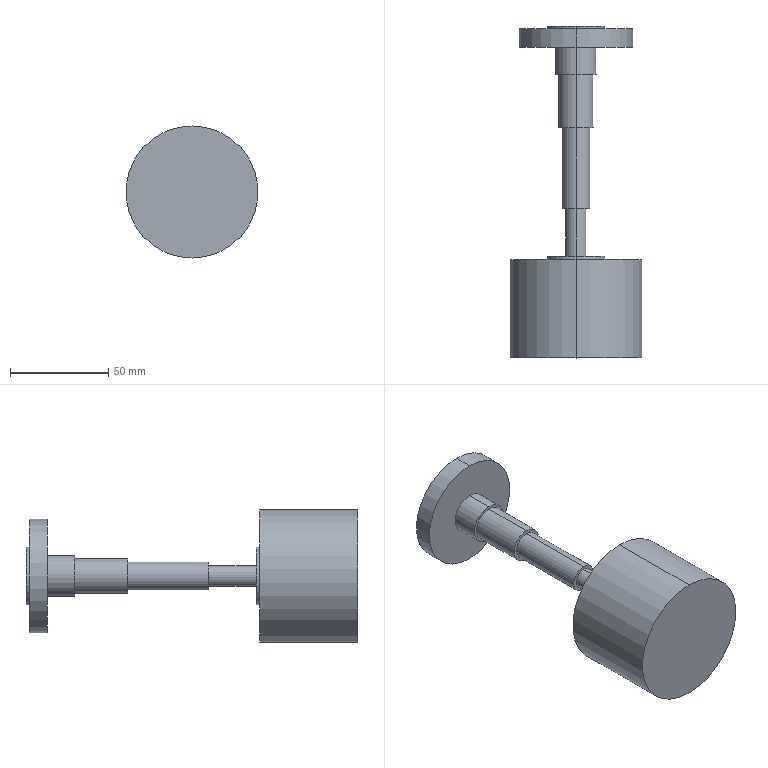Part | SolidWorks | features SavedExtBody 1 | 1 solid | 28 faces | box 67.426 x 169.265 x 67.426 mm | volume 221151 mm3 | cylinder 18 | plane 10 | commonest cylinder face diameters 29.345 x4 7.234 x2 10.656 x2 14.186 x2 17.774 x2 20.753 x2
STEP:
#1=CARTESIAN_POINT('',(0.,-304.394,79.672));
#2=VERTEX_POINT('',#1);
#3=CARTESIAN_POINT('',(0.,-304.394,50.328));
#4=VERTEX_POINT('',#3);
#5=CARTESIAN_POINT('',(0.,-304.394,65.));
#6=DIRECTION('',(0.,1.,0.));
#7=DIRECTION('',(0.,0.,1.));
#8=AXIS2_PLACEMENT_3D('',#5,#6,#7);
#9=CIRCLE('',#8,14.672);
#10=EDGE_CURVE('',#2,#4,#9,.T.);
#11=ORIENTED_EDGE('',*,*,#10,.T.);
#12=CARTESIAN_POINT('',(0.,-302.738,50.328));
#13=VERTEX_POINT('',#12);
#14=CARTESIAN_POINT('',(0.,-304.394,50.328));
#15=DIRECTION('',(0.,1.,0.));
#16=VECTOR('',#15,1000.);
#17=LINE('',#14,#16);
#18=EDGE_CURVE('',#4,#13,#17,.T.);
#19=ORIENTED_EDGE('',*,*,#18,.T.);
#20=CARTESIAN_POINT('',(0.,-302.738,79.672));
#21=VERTEX_POINT('',#20);
#22=CARTESIAN_POINT('',(0.,-302.738,65.));
#23=DIRECTION('',(0.,1.,0.));
#24=DIRECTION('',(0.,0.,1.));
#25=AXIS2_PLACEMENT_3D('',#22,#23,#24);
#26=CIRCLE('',#25,14.672);
#27=EDGE_CURVE('',#21,#13,#26,.T.);
#28=ORIENTED_EDGE('',*,*,#27,.F.);
#29=CARTESIAN_POINT('',(0.,-304.394,79.672));
#30=DIRECTION('',(0.,1.,0.));
#31=VECTOR('',#30,1000.);
#32=LINE('',#29,#31);
#33=EDGE_CURVE('',#2,#21,#32,.T.);
#34=ORIENTED_EDGE('',*,*,#33,.F.);
#35=EDGE_LOOP('',(#11,#19,#28,#34));
#36=FACE_OUTER_BOUND('',#35,.T.);
#37=CARTESIAN_POINT('',(0.,-304.394,65.));
#38=DIRECTION('',(0.,1.,0.));
#39=DIRECTION('',(0.,0.,1.));
#40=AXIS2_PLACEMENT_3D('',#37,#38,#39);
#41=CYLINDRICAL_SURFACE('',#40,14.672);
#42=ADVANCED_FACE('',(#36),#41,.T.);
#43=CARTESIAN_POINT('',(0.,-302.738,70.328));
#44=VERTEX_POINT('',#43);
#45=CARTESIAN_POINT('',(0.,-302.738,59.672));
#46=VERTEX_POINT('',#45);
#47=CARTESIAN_POINT('',(0.,-302.738,65.));
#48=DIRECTION('',(0.,1.,0.));
#49=DIRECTION('',(0.,0.,1.));
#50=AXIS2_PLACEMENT_3D('',#47,#48,#49);
#51=CIRCLE('',#50,5.328);
#52=EDGE_CURVE('',#44,#46,#51,.T.);
#53=ORIENTED_EDGE('',*,*,#52,.T.);
#54=CARTESIAN_POINT('',(0.,-278.363,59.672));
#55=VERTEX_POINT('',#54);
#56=CARTESIAN_POINT('',(0.,-304.394,59.672));
#57=DIRECTION('',(0.,1.,0.));
#58=VECTOR('',#57,1000.);
#59=LINE('',#56,#58);
#60=EDGE_CURVE('',#46,#55,#59,.T.);
#61=ORIENTED_EDGE('',*,*,#60,.T.);
#62=CARTESIAN_POINT('',(0.,-278.363,70.328));
#63=VERTEX_POINT('',#62);
#64=CARTESIAN_POINT('',(0.,-278.363,65.));
#65=DIRECTION('',(0.,1.,0.));
#66=DIRECTION('',(0.,0.,1.));
#67=AXIS2_PLACEMENT_3D('',#64,#65,#66);
#68=CIRCLE('',#67,5.328);
#69=EDGE_CURVE('',#63,#55,#68,.T.);
#70=ORIENTED_EDGE('',*,*,#69,.F.);
#71=CARTESIAN_POINT('',(0.,-304.394,70.328));
#72=DIRECTION('',(0.,1.,0.));
#73=VECTOR('',#72,1000.);
#74=LINE('',#71,#73);
#75=EDGE_CURVE('',#44,#63,#74,.T.);
#76=ORIENTED_EDGE('',*,*,#75,.F.);
#77=EDGE_LOOP('',(#53,#61,#70,#76));
#78=FACE_OUTER_BOUND('',#77,.T.);
#79=CARTESIAN_POINT('',(0.,-304.394,65.));
#80=DIRECTION('',(0.,1.,0.));
#81=DIRECTION('',(0.,0.,1.));
#82=AXIS2_PLACEMENT_3D('',#79,#80,#81);
#83=CYLINDRICAL_SURFACE('',#82,5.328);
#84=ADVANCED_FACE('',(#78),#83,.T.);
#85=CARTESIAN_POINT('',(0.,-278.363,72.093));
#86=VERTEX_POINT('',#85);
#87=CARTESIAN_POINT('',(0.,-278.363,57.907));
#88=VERTEX_POINT('',#87);
#89=CARTESIAN_POINT('',(0.,-278.363,65.));
#90=DIRECTION('',(0.,1.,0.));
#91=DIRECTION('',(0.,0.,1.));
#92=AXIS2_PLACEMENT_3D('',#89,#90,#91);
#93=CIRCLE('',#92,7.093);
#94=EDGE_CURVE('',#86,#88,#93,.T.);
#95=ORIENTED_EDGE('',*,*,#94,.T.);
#96=CARTESIAN_POINT('',(0.,-237.148,57.907));
#97=VERTEX_POINT('',#96);
#98=CARTESIAN_POINT('',(0.,-304.394,57.907));
#99=DIRECTION('',(0.,1.,0.));
#100=VECTOR('',#99,1000.);
#101=LINE('',#98,#100);
#102=EDGE_CURVE('',#88,#97,#101,.T.);
#103=ORIENTED_EDGE('',*,*,#102,.T.);
#104=CARTESIAN_POINT('',(0.,-237.148,72.093));
#105=VERTEX_POINT('',#104);
#106=CARTESIAN_POINT('',(0.,-237.148,65.));
#107=DIRECTION('',(0.,1.,0.));
#108=DIRECTION('',(0.,0.,1.));
#109=AXIS2_PLACEMENT_3D('',#106,#107,#108);
#110=CIRCLE('',#109,7.093);
#111=EDGE_CURVE('',#105,#97,#110,.T.);
#112=ORIENTED_EDGE('',*,*,#111,.F.);
#113=CARTESIAN_POINT('',(0.,-304.394,72.093));
#114=DIRECTION('',(0.,1.,0.));
#115=VECTOR('',#114,1000.);
#116=LINE('',#113,#115);
#117=EDGE_CURVE('',#86,#105,#116,.T.);
#118=ORIENTED_EDGE('',*,*,#117,.F.);
#119=EDGE_LOOP('',(#95,#103,#112,#118));
#120=FACE_OUTER_BOUND('',#119,.T.);
#121=CARTESIAN_POINT('',(0.,-304.394,65.));
#122=DIRECTION('',(0.,1.,0.));
#123=DIRECTION('',(0.,0.,1.));
#124=AXIS2_PLACEMENT_3D('',#121,#122,#123);
#125=CYLINDRICAL_SURFACE('',#124,7.093);
#126=ADVANCED_FACE('',(#120),#125,.T.);
#127=CARTESIAN_POINT('',(0.,-237.148,73.887));
#128=VERTEX_POINT('',#127);
#129=CARTESIAN_POINT('',(0.,-237.148,56.113));
#130=VERTEX_POINT('',#129);
#131=CARTESIAN_POINT('',(0.,-237.148,65.));
#132=DIRECTION('',(0.,1.,0.));
#133=DIRECTION('',(0.,0.,1.));
#134=AXIS2_PLACEMENT_3D('',#131,#132,#133);
#135=CIRCLE('',#134,8.887);
#136=EDGE_CURVE('',#128,#130,#135,.T.);
#137=ORIENTED_EDGE('',*,*,#136,.T.);
#138=CARTESIAN_POINT('',(0.,-210.021,56.113));
#139=VERTEX_POINT('',#138);
#140=CARTESIAN_POINT('',(0.,-304.394,56.113));
#141=DIRECTION('',(0.,1.,0.));
#142=VECTOR('',#141,1000.);
#143=LINE('',#140,#142);
#144=EDGE_CURVE('',#130,#139,#143,.T.);
#145=ORIENTED_EDGE('',*,*,#144,.T.);
#146=CARTESIAN_POINT('',(0.,-210.021,73.887));
#147=VERTEX_POINT('',#146);
#148=CARTESIAN_POINT('',(0.,-210.021,65.));
#149=DIRECTION('',(0.,1.,0.));
#150=DIRECTION('',(0.,0.,1.));
#151=AXIS2_PLACEMENT_3D('',#148,#149,#150);
#152=CIRCLE('',#151,8.887);
#153=EDGE_CURVE('',#147,#139,#152,.T.);
#154=ORIENTED_EDGE('',*,*,#153,.F.);
#155=CARTESIAN_POINT('',(0.,-304.394,73.887));
#156=DIRECTION('',(0.,1.,0.));
#157=VECTOR('',#156,1000.);
#158=LINE('',#155,#157);
#159=EDGE_CURVE('',#128,#147,#158,.T.);
#160=ORIENTED_EDGE('',*,*,#159,.F.);
#161=EDGE_LOOP('',(#137,#145,#154,#160));
#162=FACE_OUTER_BOUND('',#161,.T.);
#163=CARTESIAN_POINT('',(0.,-304.394,65.));
#164=DIRECTION('',(0.,1.,0.));
#165=DIRECTION('',(0.,0.,1.));
#166=AXIS2_PLACEMENT_3D('',#163,#164,#165);
#167=CYLINDRICAL_SURFACE('',#166,8.887);
#168=ADVANCED_FACE('',(#162),#167,.T.);
#169=CARTESIAN_POINT('',(0.,-210.021,75.377));
#170=VERTEX_POINT('',#169);
#171=CARTESIAN_POINT('',(0.,-210.021,54.623));
#172=VERTEX_POINT('',#171);
#173=CARTESIAN_POINT('',(0.,-210.021,65.));
#174=DIRECTION('',(0.,1.,0.));
#175=DIRECTION('',(0.,0.,1.));
#176=AXIS2_PLACEMENT_3D('',#173,#174,#175);
#177=CIRCLE('',#176,10.377);
#178=EDGE_CURVE('',#170,#172,#177,.T.);
#179=ORIENTED_EDGE('',*,*,#178,.T.);
#180=CARTESIAN_POINT('',(0.,-196.144,54.623));
#181=VERTEX_POINT('',#180);
#182=CARTESIAN_POINT('',(0.,-304.394,54.623));
#183=DIRECTION('',(0.,1.,0.));
#184=VECTOR('',#183,1000.);
#185=LINE('',#182,#184);
#186=EDGE_CURVE('',#172,#181,#185,.T.);
#187=ORIENTED_EDGE('',*,*,#186,.T.);
#188=CARTESIAN_POINT('',(0.,-196.144,75.377));
#189=VERTEX_POINT('',#188);
#190=CARTESIAN_POINT('',(0.,-196.144,65.));
#191=DIRECTION('',(0.,1.,0.));
#192=DIRECTION('',(0.,0.,1.));
#193=AXIS2_PLACEMENT_3D('',#190,#191,#192);
#194=CIRCLE('',#193,10.377);
#195=EDGE_CURVE('',#189,#181,#194,.T.);
#196=ORIENTED_EDGE('',*,*,#195,.F.);
#197=CARTESIAN_POINT('',(0.,-304.394,75.377));
#198=DIRECTION('',(0.,1.,0.));
#199=VECTOR('',#198,1000.);
#200=LINE('',#197,#199);
#201=EDGE_CURVE('',#170,#189,#200,.T.);
#202=ORIENTED_EDGE('',*,*,#201,.F.);
#203=EDGE_LOOP('',(#179,#187,#196,#202));
#204=FACE_OUTER_BOUND('',#203,.T.);
#205=CARTESIAN_POINT('',(0.,-304.394,65.));
#206=DIRECTION('',(0.,1.,0.));
#207=DIRECTION('',(0.,0.,1.));
#208=AXIS2_PLACEMENT_3D('',#205,#206,#207);
#209=CYLINDRICAL_SURFACE('',#208,10.377);
#210=ADVANCED_FACE('',(#204),#209,.T.);
#211=CARTESIAN_POINT('',(0.,-196.144,93.981));
#212=VERTEX_POINT('',#211);
#213=CARTESIAN_POINT('',(0.,-196.144,36.019));
#214=VERTEX_POINT('',#213);
#215=CARTESIAN_POINT('',(0.,-196.144,65.));
#216=DIRECTION('',(0.,1.,0.));
#217=DIRECTION('',(0.,0.,1.));
#218=AXIS2_PLACEMENT_3D('',#215,#216,#217);
#219=CIRCLE('',#218,28.981);
#220=EDGE_CURVE('',#212,#214,#219,.T.);
#221=ORIENTED_EDGE('',*,*,#220,.T.);
#222=CARTESIAN_POINT('',(0.,-186.774,36.019));
#223=VERTEX_POINT('',#222);
#224=CARTESIAN_POINT('',(0.,-304.394,36.019));
#225=DIRECTION('',(0.,1.,0.));
#226=VECTOR('',#225,1000.);
#227=LINE('',#224,#226);
#228=EDGE_CURVE('',#214,#223,#227,.T.);
#229=ORIENTED_EDGE('',*,*,#228,.T.);
#230=CARTESIAN_POINT('',(0.,-186.774,93.981));
#231=VERTEX_POINT('',#230);
#232=CARTESIAN_POINT('',(0.,-186.774,65.));
#233=DIRECTION('',(0.,1.,0.));
#234=DIRECTION('',(0.,0.,1.));
#235=AXIS2_PLACEMENT_3D('',#232,#233,#234);
#236=CIRCLE('',#235,28.981);
#237=EDGE_CURVE('',#231,#223,#236,.T.);
#238=ORIENTED_EDGE('',*,*,#237,.F.);
#239=CARTESIAN_POINT('',(0.,-304.394,93.981));
#240=DIRECTION('',(0.,1.,0.));
#241=VECTOR('',#240,1000.);
#242=LINE('',#239,#241);
#243=EDGE_CURVE('',#212,#231,#242,.T.);
#244=ORIENTED_EDGE('',*,*,#243,.F.);
#245=EDGE_LOOP('',(#221,#229,#238,#244));
#246=FACE_OUTER_BOUND('',#245,.T.);
#247=CARTESIAN_POINT('',(0.,-304.394,65.));
#248=DIRECTION('',(0.,1.,0.));
#249=DIRECTION('',(0.,0.,1.));
#250=AXIS2_PLACEMENT_3D('',#247,#248,#249);
#251=CYLINDRICAL_SURFACE('',#250,28.981);
#252=ADVANCED_FACE('',(#246),#251,.T.);
#253=CARTESIAN_POINT('',(0.,-186.774,79.672));
#254=VERTEX_POINT('',#253);
#255=CARTESIAN_POINT('',(0.,-186.774,50.328));
#256=VERTEX_POINT('',#255);
#257=CARTESIAN_POINT('',(0.,-186.774,65.));
#258=DIRECTION('',(0.,1.,0.));
#259=DIRECTION('',(0.,0.,1.));
#260=AXIS2_PLACEMENT_3D('',#257,#258,#259);
#261=CIRCLE('',#260,14.672);
#262=EDGE_CURVE('',#254,#256,#261,.T.);
#263=ORIENTED_EDGE('',*,*,#262,.T.);
#264=CARTESIAN_POINT('',(0.,-185.285,50.328));
#265=VERTEX_POINT('',#264);
#266=CARTESIAN_POINT('',(0.,-304.394,50.328));
#267=DIRECTION('',(0.,1.,0.));
#268=VECTOR('',#267,1000.);
#269=LINE('',#266,#268);
#270=EDGE_CURVE('',#256,#265,#269,.T.);
#271=ORIENTED_EDGE('',*,*,#270,.T.);
#272=CARTESIAN_POINT('',(0.,-185.285,79.672));
#273=VERTEX_POINT('',#272);
#274=CARTESIAN_POINT('',(0.,-185.285,65.));
#275=DIRECTION('',(0.,1.,0.));
#276=DIRECTION('',(0.,0.,1.));
#277=AXIS2_PLACEMENT_3D('',#274,#275,#276);
#278=CIRCLE('',#277,14.672);
#279=EDGE_CURVE('',#273,#265,#278,.T.);
#280=ORIENTED_EDGE('',*,*,#279,.F.);
#281=CARTESIAN_POINT('',(0.,-304.394,79.672));
#282=DIRECTION('',(0.,1.,0.));
#283=VECTOR('',#282,1000.);
#284=LINE('',#281,#283);
#285=EDGE_CURVE('',#254,#273,#284,.T.);
#286=ORIENTED_EDGE('',*,*,#285,.F.);
#287=EDGE_LOOP('',(#263,#271,#280,#286));
#288=FACE_OUTER_BOUND('',#287,.T.);
#289=CARTESIAN_POINT('',(0.,-304.394,65.));
#290=DIRECTION('',(0.,1.,0.));
#291=DIRECTION('',(0.,0.,1.));
#292=AXIS2_PLACEMENT_3D('',#289,#290,#291);
#293=CYLINDRICAL_SURFACE('',#292,14.672);
#294=ADVANCED_FACE('',(#288),#293,.T.);
#295=CARTESIAN_POINT('',(0.,-304.394,61.383));
#296=VERTEX_POINT('',#295);
#297=CARTESIAN_POINT('',(0.,-304.394,68.617));
#298=VERTEX_POINT('',#297);
#299=CARTESIAN_POINT('',(0.,-304.394,65.));
#300=DIRECTION('',(0.,1.,0.));
#301=DIRECTION('',(0.,0.,1.));
#302=AXIS2_PLACEMENT_3D('',#299,#300,#301);
#303=CIRCLE('',#302,3.617);
#304=EDGE_CURVE('',#296,#298,#303,.T.);
#305=ORIENTED_EDGE('',*,*,#304,.F.);
#306=CARTESIAN_POINT('',(0.,-185.285,61.383));
#307=VERTEX_POINT('',#306);
#308=CARTESIAN_POINT('',(0.,-304.394,61.383));
#309=DIRECTION('',(0.,1.,0.));
#310=VECTOR('',#309,1000.);
#311=LINE('',#308,#310);
#312=EDGE_CURVE('',#296,#307,#311,.T.);
#313=ORIENTED_EDGE('',*,*,#312,.T.);
#314=CARTESIAN_POINT('',(0.,-185.285,68.617));
#315=VERTEX_POINT('',#314);
#316=CARTESIAN_POINT('',(0.,-185.285,65.));
#317=DIRECTION('',(0.,1.,0.));
#318=DIRECTION('',(0.,0.,1.));
#319=AXIS2_PLACEMENT_3D('',#316,#317,#318);
#320=CIRCLE('',#319,3.617);
#321=EDGE_CURVE('',#307,#315,#320,.T.);
#322=ORIENTED_EDGE('',*,*,#321,.T.);
#323=CARTESIAN_POINT('',(0.,-304.394,68.617));
#324=DIRECTION('',(0.,1.,0.));
#325=VECTOR('',#324,1000.);
#326=LINE('',#323,#325);
#327=EDGE_CURVE('',#298,#315,#326,.T.);
#328=ORIENTED_EDGE('',*,*,#327,.F.);
#329=EDGE_LOOP('',(#305,#313,#322,#328));
#330=FACE_OUTER_BOUND('',#329,.T.);
#331=CARTESIAN_POINT('',(0.,-304.394,65.));
#332=DIRECTION('',(0.,1.,0.));
#333=DIRECTION('',(0.,0.,1.));
#334=AXIS2_PLACEMENT_3D('',#331,#332,#333);
#335=CYLINDRICAL_SURFACE('',#334,3.617);
#336=ADVANCED_FACE('',(#330),#335,.F.);
#337=CARTESIAN_POINT('',(0.,-354.549,98.713));
#338=VERTEX_POINT('',#337);
#339=CARTESIAN_POINT('',(0.,-354.549,31.287));
#340=VERTEX_POINT('',#339);
#341=CARTESIAN_POINT('',(0.,-354.549,65.));
#342=DIRECTION('',(0.,1.,0.));
#343=DIRECTION('',(0.,0.,1.));
#344=AXIS2_PLACEMENT_3D('',#341,#342,#343);
#345=CIRCLE('',#344,33.713);
#346=EDGE_CURVE('',#338,#340,#345,.T.);
#347=ORIENTED_EDGE('',*,*,#346,.T.);
#348=CARTESIAN_POINT('',(0.,-304.394,31.287));
#349=VERTEX_POINT('',#348);
#350=CARTESIAN_POINT('',(0.,-304.394,31.287));
#351=DIRECTION('',(0.,1.,0.));
#352=VECTOR('',#351,1000.);
#353=LINE('',#350,#352);
#354=EDGE_CURVE('',#340,#349,#353,.T.);
#355=ORIENTED_EDGE('',*,*,#354,.T.);
#356=CARTESIAN_POINT('',(0.,-304.394,98.713));
#357=VERTEX_POINT('',#356);
#358=CARTESIAN_POINT('',(0.,-304.394,65.));
#359=DIRECTION('',(0.,1.,0.));
#360=DIRECTION('',(0.,0.,1.));
#361=AXIS2_PLACEMENT_3D('',#358,#359,#360);
#362=CIRCLE('',#361,33.713);
#363=EDGE_CURVE('',#357,#349,#362,.T.);
#364=ORIENTED_EDGE('',*,*,#363,.F.);
#365=CARTESIAN_POINT('',(0.,-304.394,98.713));
#366=DIRECTION('',(0.,1.,0.));
#367=VECTOR('',#366,1000.);
#368=LINE('',#365,#367);
#369=EDGE_CURVE('',#338,#357,#368,.T.);
#370=ORIENTED_EDGE('',*,*,#369,.F.);
#371=EDGE_LOOP('',(#347,#355,#364,#370));
#372=FACE_OUTER_BOUND('',#371,.T.);
#373=CARTESIAN_POINT('',(0.,-304.394,65.));
#374=DIRECTION('',(0.,1.,0.));
#375=DIRECTION('',(0.,0.,1.));
#376=AXIS2_PLACEMENT_3D('',#373,#374,#375);
#377=CYLINDRICAL_SURFACE('',#376,33.713);
#378=ADVANCED_FACE('',(#372),#377,.T.);
#379=ORIENTED_EDGE('',*,*,#354,.F.);
#380=CARTESIAN_POINT('',(0.,-354.549,65.));
#381=DIRECTION('',(0.,1.,0.));
#382=DIRECTION('',(0.,0.,1.));
#383=AXIS2_PLACEMENT_3D('',#380,#381,#382);
#384=CIRCLE('',#383,33.713);
#385=EDGE_CURVE('',#340,#338,#384,.T.);
#386=ORIENTED_EDGE('',*,*,#385,.T.);
#387=ORIENTED_EDGE('',*,*,#369,.T.);
#388=CARTESIAN_POINT('',(0.,-304.394,65.));
#389=DIRECTION('',(0.,1.,0.));
#390=DIRECTION('',(0.,0.,1.));
#391=AXIS2_PLACEMENT_3D('',#388,#389,#390);
#392=CIRCLE('',#391,33.713);
#393=EDGE_CURVE('',#349,#357,#392,.T.);
#394=ORIENTED_EDGE('',*,*,#393,.F.);
#395=EDGE_LOOP('',(#379,#386,#387,#394));
#396=FACE_OUTER_BOUND('',#395,.T.);
#397=CARTESIAN_POINT('',(0.,-304.394,65.));
#398=DIRECTION('',(0.,1.,0.));
#399=DIRECTION('',(0.,0.,1.));
#400=AXIS2_PLACEMENT_3D('',#397,#398,#399);
#401=CYLINDRICAL_SURFACE('',#400,33.713);
#402=ADVANCED_FACE('',(#396),#401,.T.);
#403=ORIENTED_EDGE('',*,*,#346,.F.);
#404=ORIENTED_EDGE('',*,*,#385,.F.);
#405=EDGE_LOOP('',(#403,#404));
#406=FACE_OUTER_BOUND('',#405,.T.);
#407=CARTESIAN_POINT('',(-33.713,-354.549,65.));
#408=DIRECTION('',(0.,-1.,0.));
#409=DIRECTION('',(0.,0.,-1.));
#410=AXIS2_PLACEMENT_3D('',#407,#408,#409);
#411=PLANE('',#410);
#412=ADVANCED_FACE('',(#406),#411,.T.);
#413=CARTESIAN_POINT('',(0.,-304.394,65.));
#414=DIRECTION('',(0.,1.,0.));
#415=DIRECTION('',(0.,0.,1.));
#416=AXIS2_PLACEMENT_3D('',#413,#414,#415);
#417=CIRCLE('',#416,3.617);
#418=EDGE_CURVE('',#298,#296,#417,.T.);
#419=ORIENTED_EDGE('',*,*,#418,.T.);
#420=ORIENTED_EDGE('',*,*,#304,.T.);
#421=EDGE_LOOP('',(#419,#420));
#422=FACE_OUTER_BOUND('',#421,.T.);
#423=CARTESIAN_POINT('',(-3.617,-304.394,65.));
#424=DIRECTION('',(0.,1.,0.));
#425=DIRECTION('',(0.,0.,1.));
#426=AXIS2_PLACEMENT_3D('',#423,#424,#425);
#427=PLANE('',#426);
#428=ADVANCED_FACE('',(#422),#427,.T.);
#429=ORIENTED_EDGE('',*,*,#312,.F.);
#430=ORIENTED_EDGE('',*,*,#418,.F.);
#431=ORIENTED_EDGE('',*,*,#327,.T.);
#432=CARTESIAN_POINT('',(0.,-185.285,65.));
#433=DIRECTION('',(0.,1.,0.));
#434=DIRECTION('',(0.,0.,1.));
#435=AXIS2_PLACEMENT_3D('',#432,#433,#434);
#436=CIRCLE('',#435,3.617);
#437=EDGE_CURVE('',#315,#307,#436,.T.);
#438=ORIENTED_EDGE('',*,*,#437,.T.);
#439=EDGE_LOOP('',(#429,#430,#431,#438));
#440=FACE_OUTER_BOUND('',#439,.T.);
#441=CARTESIAN_POINT('',(0.,-304.394,65.));
#442=DIRECTION('',(0.,1.,0.));
#443=DIRECTION('',(0.,0.,1.));
#444=AXIS2_PLACEMENT_3D('',#441,#442,#443);
#445=CYLINDRICAL_SURFACE('',#444,3.617);
#446=ADVANCED_FACE('',(#440),#445,.F.);
#447=ORIENTED_EDGE('',*,*,#279,.T.);
#448=CARTESIAN_POINT('',(0.,-185.285,65.));
#449=DIRECTION('',(0.,1.,0.));
#450=DIRECTION('',(0.,0.,1.));
#451=AXIS2_PLACEMENT_3D('',#448,#449,#450);
#452=CIRCLE('',#451,14.672);
#453=EDGE_CURVE('',#265,#273,#452,.T.);
#454=ORIENTED_EDGE('',*,*,#453,.T.);
#455=EDGE_LOOP('',(#447,#454));
#456=FACE_OUTER_BOUND('',#455,.T.);
#457=ORIENTED_EDGE('',*,*,#437,.F.);
#458=ORIENTED_EDGE('',*,*,#321,.F.);
#459=EDGE_LOOP('',(#457,#458));
#460=FACE_BOUND('',#459,.T.);
#461=CARTESIAN_POINT('',(-12.5,-185.285,65.));
#462=DIRECTION('',(0.,1.,0.));
#463=DIRECTION('',(0.,0.,1.));
#464=AXIS2_PLACEMENT_3D('',#461,#462,#463);
#465=PLANE('',#464);
#466=ADVANCED_FACE('',(#456,#460),#465,.T.);
#467=ORIENTED_EDGE('',*,*,#270,.F.);
#468=CARTESIAN_POINT('',(0.,-186.774,65.));
#469=DIRECTION('',(0.,1.,0.));
#470=DIRECTION('',(0.,0.,1.));
#471=AXIS2_PLACEMENT_3D('',#468,#469,#470);
#472=CIRCLE('',#471,14.672);
#473=EDGE_CURVE('',#256,#254,#472,.T.);
#474=ORIENTED_EDGE('',*,*,#473,.T.);
#475=ORIENTED_EDGE('',*,*,#285,.T.);
#476=ORIENTED_EDGE('',*,*,#453,.F.);
#477=EDGE_LOOP('',(#467,#474,#475,#476));
#478=FACE_OUTER_BOUND('',#477,.T.);
#479=CARTESIAN_POINT('',(0.,-304.394,65.));
#480=DIRECTION('',(0.,1.,0.));
#481=DIRECTION('',(0.,0.,1.));
#482=AXIS2_PLACEMENT_3D('',#479,#480,#481);
#483=CYLINDRICAL_SURFACE('',#482,14.672);
#484=ADVANCED_FACE('',(#478),#483,.T.);
#485=ORIENTED_EDGE('',*,*,#237,.T.);
#486=CARTESIAN_POINT('',(0.,-186.774,65.));
#487=DIRECTION('',(0.,1.,0.));
#488=DIRECTION('',(0.,0.,1.));
#489=AXIS2_PLACEMENT_3D('',#486,#487,#488);
#490=CIRCLE('',#489,28.981);
#491=EDGE_CURVE('',#223,#231,#490,.T.);
#492=ORIENTED_EDGE('',*,*,#491,.T.);
#493=EDGE_LOOP('',(#485,#492));
#494=FACE_OUTER_BOUND('',#493,.T.);
#495=ORIENTED_EDGE('',*,*,#262,.F.);
#496=ORIENTED_EDGE('',*,*,#473,.F.);
#497=EDGE_LOOP('',(#495,#496));
#498=FACE_BOUND('',#497,.T.);
#499=CARTESIAN_POINT('',(-14.672,-186.774,65.));
#500=DIRECTION('',(0.,1.,0.));
#501=DIRECTION('',(0.,0.,1.));
#502=AXIS2_PLACEMENT_3D('',#499,#500,#501);
#503=PLANE('',#502);
#504=ADVANCED_FACE('',(#494,#498),#503,.T.);
#505=ORIENTED_EDGE('',*,*,#228,.F.);
#506=CARTESIAN_POINT('',(0.,-196.144,65.));
#507=DIRECTION('',(0.,1.,0.));
#508=DIRECTION('',(0.,0.,1.));
#509=AXIS2_PLACEMENT_3D('',#506,#507,#508);
#510=CIRCLE('',#509,28.981);
#511=EDGE_CURVE('',#214,#212,#510,.T.);
#512=ORIENTED_EDGE('',*,*,#511,.T.);
#513=ORIENTED_EDGE('',*,*,#243,.T.);
#514=ORIENTED_EDGE('',*,*,#491,.F.);
#515=EDGE_LOOP('',(#505,#512,#513,#514));
#516=FACE_OUTER_BOUND('',#515,.T.);
#517=CARTESIAN_POINT('',(0.,-304.394,65.));
#518=DIRECTION('',(0.,1.,0.));
#519=DIRECTION('',(0.,0.,1.));
#520=AXIS2_PLACEMENT_3D('',#517,#518,#519);
#521=CYLINDRICAL_SURFACE('',#520,28.981);
#522=ADVANCED_FACE('',(#516),#521,.T.);
#523=ORIENTED_EDGE('',*,*,#195,.T.);
#524=CARTESIAN_POINT('',(0.,-196.144,65.));
#525=DIRECTION('',(0.,1.,0.));
#526=DIRECTION('',(0.,0.,1.));
#527=AXIS2_PLACEMENT_3D('',#524,#525,#526);
#528=CIRCLE('',#527,10.377);
#529=EDGE_CURVE('',#181,#189,#528,.T.);
#530=ORIENTED_EDGE('',*,*,#529,.T.);
#531=EDGE_LOOP('',(#523,#530));
#532=FACE_BOUND('',#531,.T.);
#533=ORIENTED_EDGE('',*,*,#220,.F.);
#534=ORIENTED_EDGE('',*,*,#511,.F.);
#535=EDGE_LOOP('',(#533,#534));
#536=FACE_OUTER_BOUND('',#535,.T.);
#537=CARTESIAN_POINT('',(-28.981,-196.144,65.));
#538=DIRECTION('',(0.,-1.,0.));
#539=DIRECTION('',(0.,0.,-1.));
#540=AXIS2_PLACEMENT_3D('',#537,#538,#539);
#541=PLANE('',#540);
#542=ADVANCED_FACE('',(#532,#536),#541,.T.);
#543=ORIENTED_EDGE('',*,*,#186,.F.);
#544=CARTESIAN_POINT('',(0.,-210.021,65.));
#545=DIRECTION('',(0.,1.,0.));
#546=DIRECTION('',(0.,0.,1.));
#547=AXIS2_PLACEMENT_3D('',#544,#545,#546);
#548=CIRCLE('',#547,10.377);
#549=EDGE_CURVE('',#172,#170,#548,.T.);
#550=ORIENTED_EDGE('',*,*,#549,.T.);
#551=ORIENTED_EDGE('',*,*,#201,.T.);
#552=ORIENTED_EDGE('',*,*,#529,.F.);
#553=EDGE_LOOP('',(#543,#550,#551,#552));
#554=FACE_OUTER_BOUND('',#553,.T.);
#555=CARTESIAN_POINT('',(0.,-304.394,65.));
#556=DIRECTION('',(0.,1.,0.));
#557=DIRECTION('',(0.,0.,1.));
#558=AXIS2_PLACEMENT_3D('',#555,#556,#557);
#559=CYLINDRICAL_SURFACE('',#558,10.377);
#560=ADVANCED_FACE('',(#554),#559,.T.);
#561=ORIENTED_EDGE('',*,*,#153,.T.);
#562=CARTESIAN_POINT('',(0.,-210.021,65.));
#563=DIRECTION('',(0.,1.,0.));
#564=DIRECTION('',(0.,0.,1.));
#565=AXIS2_PLACEMENT_3D('',#562,#563,#564);
#566=CIRCLE('',#565,8.887);
#567=EDGE_CURVE('',#139,#147,#566,.T.);
#568=ORIENTED_EDGE('',*,*,#567,.T.);
#569=EDGE_LOOP('',(#561,#568));
#570=FACE_BOUND('',#569,.T.);
#571=ORIENTED_EDGE('',*,*,#178,.F.);
#572=ORIENTED_EDGE('',*,*,#549,.F.);
#573=EDGE_LOOP('',(#571,#572));
#574=FACE_OUTER_BOUND('',#573,.T.);
#575=CARTESIAN_POINT('',(-10.377,-210.021,65.));
#576=DIRECTION('',(0.,-1.,0.));
#577=DIRECTION('',(0.,0.,-1.));
#578=AXIS2_PLACEMENT_3D('',#575,#576,#577);
#579=PLANE('',#578);
#580=ADVANCED_FACE('',(#570,#574),#579,.T.);
#581=ORIENTED_EDGE('',*,*,#144,.F.);
#582=CARTESIAN_POINT('',(0.,-237.148,65.));
#583=DIRECTION('',(0.,1.,0.));
#584=DIRECTION('',(0.,0.,1.));
#585=AXIS2_PLACEMENT_3D('',#582,#583,#584);
#586=CIRCLE('',#585,8.887);
#587=EDGE_CURVE('',#130,#128,#586,.T.);
#588=ORIENTED_EDGE('',*,*,#587,.T.);
#589=ORIENTED_EDGE('',*,*,#159,.T.);
#590=ORIENTED_EDGE('',*,*,#567,.F.);
#591=EDGE_LOOP('',(#581,#588,#589,#590));
#592=FACE_OUTER_BOUND('',#591,.T.);
#593=CARTESIAN_POINT('',(0.,-304.394,65.));
#594=DIRECTION('',(0.,1.,0.));
#595=DIRECTION('',(0.,0.,1.));
#596=AXIS2_PLACEMENT_3D('',#593,#594,#595);
#597=CYLINDRICAL_SURFACE('',#596,8.887);
#598=ADVANCED_FACE('',(#592),#597,.T.);
#599=ORIENTED_EDGE('',*,*,#111,.T.);
#600=CARTESIAN_POINT('',(0.,-237.148,65.));
#601=DIRECTION('',(0.,1.,0.));
#602=DIRECTION('',(0.,0.,1.));
#603=AXIS2_PLACEMENT_3D('',#600,#601,#602);
#604=CIRCLE('',#603,7.093);
#605=EDGE_CURVE('',#97,#105,#604,.T.);
#606=ORIENTED_EDGE('',*,*,#605,.T.);
#607=EDGE_LOOP('',(#599,#606));
#608=FACE_BOUND('',#607,.T.);
#609=ORIENTED_EDGE('',*,*,#136,.F.);
#610=ORIENTED_EDGE('',*,*,#587,.F.);
#611=EDGE_LOOP('',(#609,#610));
#612=FACE_OUTER_BOUND('',#611,.T.);
#613=CARTESIAN_POINT('',(-8.887,-237.148,65.));
#614=DIRECTION('',(0.,-1.,0.));
#615=DIRECTION('',(0.,0.,-1.));
#616=AXIS2_PLACEMENT_3D('',#613,#614,#615);
#617=PLANE('',#616);
#618=ADVANCED_FACE('',(#608,#612),#617,.T.);
#619=ORIENTED_EDGE('',*,*,#102,.F.);
#620=CARTESIAN_POINT('',(0.,-278.363,65.));
#621=DIRECTION('',(0.,1.,0.));
#622=DIRECTION('',(0.,0.,1.));
#623=AXIS2_PLACEMENT_3D('',#620,#621,#622);
#624=CIRCLE('',#623,7.093);
#625=EDGE_CURVE('',#88,#86,#624,.T.);
#626=ORIENTED_EDGE('',*,*,#625,.T.);
#627=ORIENTED_EDGE('',*,*,#117,.T.);
#628=ORIENTED_EDGE('',*,*,#605,.F.);
#629=EDGE_LOOP('',(#619,#626,#627,#628));
#630=FACE_OUTER_BOUND('',#629,.T.);
#631=CARTESIAN_POINT('',(0.,-304.394,65.));
#632=DIRECTION('',(0.,1.,0.));
#633=DIRECTION('',(0.,0.,1.));
#634=AXIS2_PLACEMENT_3D('',#631,#632,#633);
#635=CYLINDRICAL_SURFACE('',#634,7.093);
#636=ADVANCED_FACE('',(#630),#635,.T.);
#637=ORIENTED_EDGE('',*,*,#69,.T.);
#638=CARTESIAN_POINT('',(0.,-278.363,65.));
#639=DIRECTION('',(0.,1.,0.));
#640=DIRECTION('',(0.,0.,1.));
#641=AXIS2_PLACEMENT_3D('',#638,#639,#640);
#642=CIRCLE('',#641,5.328);
#643=EDGE_CURVE('',#55,#63,#642,.T.);
#644=ORIENTED_EDGE('',*,*,#643,.T.);
#645=EDGE_LOOP('',(#637,#644));
#646=FACE_BOUND('',#645,.T.);
#647=ORIENTED_EDGE('',*,*,#94,.F.);
#648=ORIENTED_EDGE('',*,*,#625,.F.);
#649=EDGE_LOOP('',(#647,#648));
#650=FACE_OUTER_BOUND('',#649,.T.);
#651=CARTESIAN_POINT('',(-7.093,-278.363,65.));
#652=DIRECTION('',(0.,-1.,0.));
#653=DIRECTION('',(0.,0.,-1.));
#654=AXIS2_PLACEMENT_3D('',#651,#652,#653);
#655=PLANE('',#654);
#656=ADVANCED_FACE('',(#646,#650),#655,.T.);
#657=ORIENTED_EDGE('',*,*,#60,.F.);
#658=CARTESIAN_POINT('',(0.,-302.738,65.));
#659=DIRECTION('',(0.,1.,0.));
#660=DIRECTION('',(0.,0.,1.));
#661=AXIS2_PLACEMENT_3D('',#658,#659,#660);
#662=CIRCLE('',#661,5.328);
#663=EDGE_CURVE('',#46,#44,#662,.T.);
#664=ORIENTED_EDGE('',*,*,#663,.T.);
#665=ORIENTED_EDGE('',*,*,#75,.T.);
#666=ORIENTED_EDGE('',*,*,#643,.F.);
#667=EDGE_LOOP('',(#657,#664,#665,#666));
#668=FACE_OUTER_BOUND('',#667,.T.);
#669=CARTESIAN_POINT('',(0.,-304.394,65.));
#670=DIRECTION('',(0.,1.,0.));
#671=DIRECTION('',(0.,0.,1.));
#672=AXIS2_PLACEMENT_3D('',#669,#670,#671);
#673=CYLINDRICAL_SURFACE('',#672,5.328);
#674=ADVANCED_FACE('',(#668),#673,.T.);
#675=ORIENTED_EDGE('',*,*,#27,.T.);
#676=CARTESIAN_POINT('',(0.,-302.738,65.));
#677=DIRECTION('',(0.,1.,0.));
#678=DIRECTION('',(0.,0.,1.));
#679=AXIS2_PLACEMENT_3D('',#676,#677,#678);
#680=CIRCLE('',#679,14.672);
#681=EDGE_CURVE('',#13,#21,#680,.T.);
#682=ORIENTED_EDGE('',*,*,#681,.T.);
#683=EDGE_LOOP('',(#675,#682));
#684=FACE_OUTER_BOUND('',#683,.T.);
#685=ORIENTED_EDGE('',*,*,#52,.F.);
#686=ORIENTED_EDGE('',*,*,#663,.F.);
#687=EDGE_LOOP('',(#685,#686));
#688=FACE_BOUND('',#687,.T.);
#689=CARTESIAN_POINT('',(-5.328,-302.738,65.));
#690=DIRECTION('',(0.,1.,0.));
#691=DIRECTION('',(0.,0.,1.));
#692=AXIS2_PLACEMENT_3D('',#689,#690,#691);
#693=PLANE('',#692);
#694=ADVANCED_FACE('',(#684,#688),#693,.T.);
#695=ORIENTED_EDGE('',*,*,#18,.F.);
#696=CARTESIAN_POINT('',(0.,-304.394,65.));
#697=DIRECTION('',(0.,1.,0.));
#698=DIRECTION('',(0.,0.,1.));
#699=AXIS2_PLACEMENT_3D('',#696,#697,#698);
#700=CIRCLE('',#699,14.672);
#701=EDGE_CURVE('',#4,#2,#700,.T.);
#702=ORIENTED_EDGE('',*,*,#701,.T.);
#703=ORIENTED_EDGE('',*,*,#33,.T.);
#704=ORIENTED_EDGE('',*,*,#681,.F.);
#705=EDGE_LOOP('',(#695,#702,#703,#704));
#706=FACE_OUTER_BOUND('',#705,.T.);
#707=CARTESIAN_POINT('',(0.,-304.394,65.));
#708=DIRECTION('',(0.,1.,0.));
#709=DIRECTION('',(0.,0.,1.));
#710=AXIS2_PLACEMENT_3D('',#707,#708,#709);
#711=CYLINDRICAL_SURFACE('',#710,14.672);
#712=ADVANCED_FACE('',(#706),#711,.T.);
#713=ORIENTED_EDGE('',*,*,#363,.T.);
#714=ORIENTED_EDGE('',*,*,#393,.T.);
#715=EDGE_LOOP('',(#713,#714));
#716=FACE_OUTER_BOUND('',#715,.T.);
#717=ORIENTED_EDGE('',*,*,#10,.F.);
#718=ORIENTED_EDGE('',*,*,#701,.F.);
#719=EDGE_LOOP('',(#717,#718));
#720=FACE_BOUND('',#719,.T.);
#721=CARTESIAN_POINT('',(-33.713,-304.394,65.));
#722=DIRECTION('',(0.,1.,0.));
#723=DIRECTION('',(0.,0.,1.));
#724=AXIS2_PLACEMENT_3D('',#721,#722,#723);
#725=PLANE('',#724);
#726=ADVANCED_FACE('',(#716,#720),#725,.T.);
#727=CLOSED_SHELL('',(#42,#84,#126,#168,#210,#252,#294,#336,#378,#402,#412,#428,#446,#466,#484,#504,#522,#542,#560,#580,#598,#618,#636,#656,#674,#694,#712,#726));
#728=MANIFOLD_SOLID_BREP('',#727);
#729=CARTESIAN_POINT('',(0.,0.,0.));
#730=DIRECTION('',(0.,0.,1.));
#731=DIRECTION('',(1.,0.,0.));
#732=AXIS2_PLACEMENT_3D('',#729,#730,#731);
#733=(LENGTH_UNIT()NAMED_UNIT(*)SI_UNIT(.MILLI.,.METRE.));
#734=UNCERTAINTY_MEASURE_WITH_UNIT(LENGTH_MEASURE(0.00001),#733,'','');
#735=(NAMED_UNIT(*)PLANE_ANGLE_UNIT()SI_UNIT($,.RADIAN.));
#736=(NAMED_UNIT(*)SI_UNIT($,.STERADIAN.)SOLID_ANGLE_UNIT());
#737=(GEOMETRIC_REPRESENTATION_CONTEXT(3)GLOBAL_UNCERTAINTY_ASSIGNED_CONTEXT((#734))GLOBAL_UNIT_ASSIGNED_CONTEXT((#733,#735,#736))REPRESENTATION_CONTEXT('',''));
#738=ADVANCED_BREP_SHAPE_REPRESENTATION('',(#728,#732),#737);